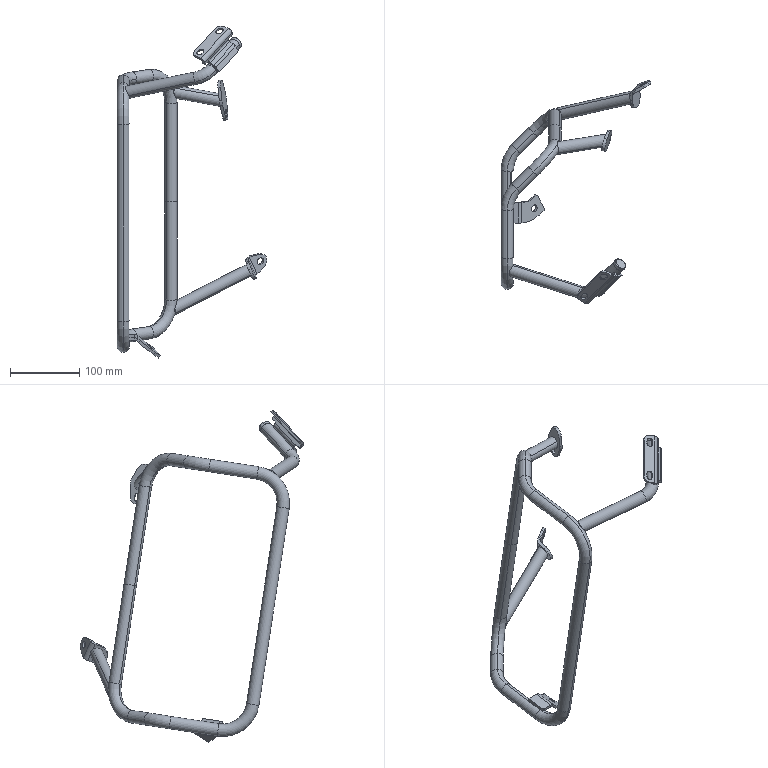Part | SolidWorks | 9 solids | 284 faces | box 216.688 x 323.225 x 479.984 mm | volume 180446 mm3 | cylinder 116 | plane 100 | torus 34 | spline 30 | cone 4 | commonest cylinder face diameters 14 x24 18 x24 9.1 x14 8 x8 6 x7 4 x6